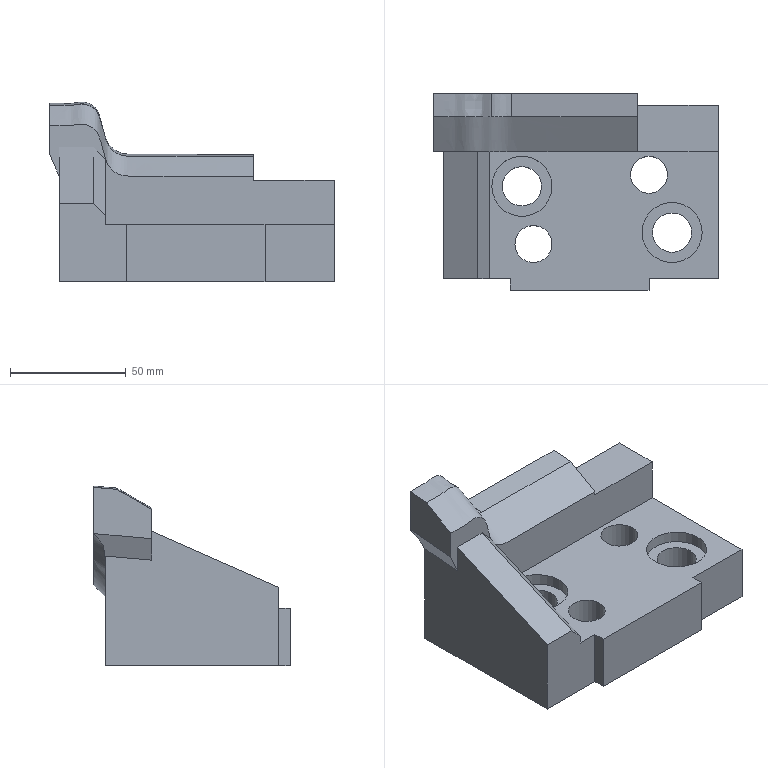Part | NX | features solid 2 | 1 solid | 32 faces | box 123.182 x 85 x 77.85 mm | volume 307666 mm3 | plane 21 | cylinder 6 | spline 5 | commonest cylinder face diameters 16 x2 17 x2 26 x2